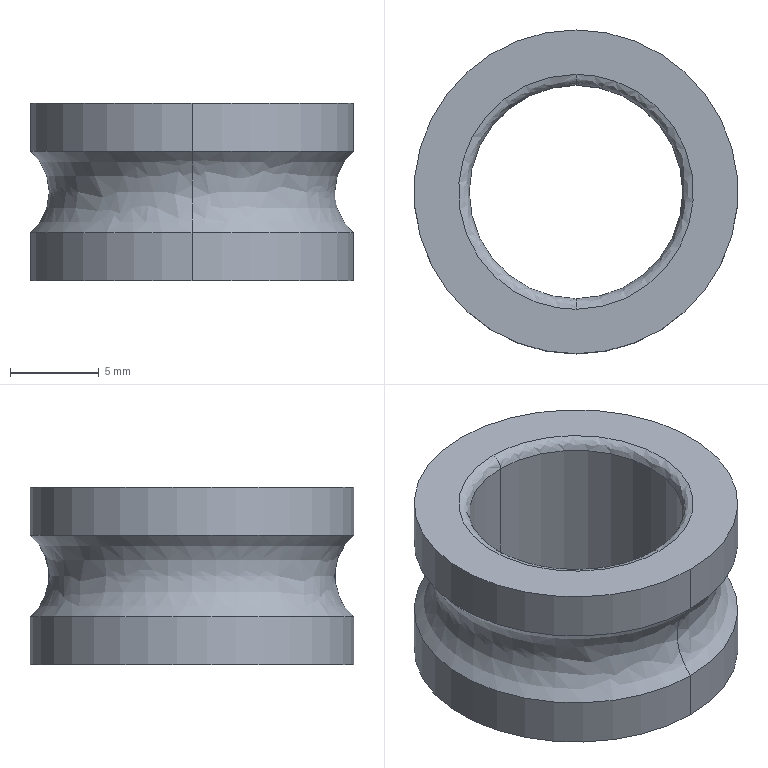Part | SolidWorks | features BaseBody 1 | 1 solid | 14 faces | box 18.2 x 18.2 x 10 mm | volume 1277 mm3 | spline 6 | cylinder 6 | plane 2 | commonest cylinder face diameters 18.2 x4 12 x2
STEP:
#1=CARTESIAN_POINT('',(0.,6.6,10.));
#2=VERTEX_POINT('',#1);
#3=CARTESIAN_POINT('',(0.,-6.6,10.));
#4=VERTEX_POINT('',#3);
#5=CARTESIAN_POINT('',(0.,6.6,10.));
#6=CARTESIAN_POINT('',(-13.2,6.6,10.));
#7=CARTESIAN_POINT('',(-13.2,-6.6,10.));
#8=CARTESIAN_POINT('',(0.,-6.6,10.));
#9=(BOUNDED_CURVE()B_SPLINE_CURVE(3,(#5,#6,#7,#8),.UNSPECIFIED.,.F.,.F.)B_SPLINE_CURVE_WITH_KNOTS((4,4),(0.25,0.75),.UNSPECIFIED.)CURVE()GEOMETRIC_REPRESENTATION_ITEM()RATIONAL_B_SPLINE_CURVE((1.,0.3333,0.3333,1.))REPRESENTATION_ITEM(''));
#10=EDGE_CURVE('',#2,#4,#9,.T.);
#11=ORIENTED_EDGE('',*,*,#10,.T.);
#12=CARTESIAN_POINT('',(0.,-6.,9.4));
#13=VERTEX_POINT('',#12);
#14=CARTESIAN_POINT('',(0.,-6.6,9.4));
#15=DIRECTION('',(-1.,0.,0.));
#16=DIRECTION('',(0.,-1.,0.));
#17=AXIS2_PLACEMENT_3D('',#14,#15,#16);
#18=CIRCLE('',#17,0.6);
#19=EDGE_CURVE('',#4,#13,#18,.T.);
#20=ORIENTED_EDGE('',*,*,#19,.T.);
#21=CARTESIAN_POINT('',(0.,6.,9.4));
#22=VERTEX_POINT('',#21);
#23=CARTESIAN_POINT('',(0.,0.,9.4));
#24=DIRECTION('',(0.,0.,-1.));
#25=DIRECTION('',(0.,1.,0.));
#26=AXIS2_PLACEMENT_3D('',#23,#24,#25);
#27=CIRCLE('',#26,6.);
#28=EDGE_CURVE('',#13,#22,#27,.T.);
#29=ORIENTED_EDGE('',*,*,#28,.T.);
#30=CARTESIAN_POINT('',(0.,6.6,9.4));
#31=DIRECTION('',(1.,0.,0.));
#32=DIRECTION('',(0.,1.,0.));
#33=AXIS2_PLACEMENT_3D('',#30,#31,#32);
#34=CIRCLE('',#33,0.6);
#35=EDGE_CURVE('',#2,#22,#34,.T.);
#36=ORIENTED_EDGE('',*,*,#35,.F.);
#37=EDGE_LOOP('',(#11,#20,#29,#36));
#38=FACE_OUTER_BOUND('',#37,.T.);
#39=CARTESIAN_POINT('',(0.,-6.6,10.));
#40=CARTESIAN_POINT('',(-13.2,-6.6,10.));
#41=CARTESIAN_POINT('',(-13.2,6.6,10.));
#42=CARTESIAN_POINT('',(0.,6.6,10.));
#43=CARTESIAN_POINT('',(0.,-6.249,10.));
#44=CARTESIAN_POINT('',(-12.497,-6.249,10.));
#45=CARTESIAN_POINT('',(-12.497,6.249,10.));
#46=CARTESIAN_POINT('',(0.,6.249,10.));
#47=CARTESIAN_POINT('',(0.,-6.,9.751));
#48=CARTESIAN_POINT('',(-12.,-6.,9.751));
#49=CARTESIAN_POINT('',(-12.,6.,9.751));
#50=CARTESIAN_POINT('',(0.,6.,9.751));
#51=CARTESIAN_POINT('',(0.,-6.,9.4));
#52=CARTESIAN_POINT('',(-12.,-6.,9.4));
#53=CARTESIAN_POINT('',(-12.,6.,9.4));
#54=CARTESIAN_POINT('',(0.,6.,9.4));
#55=(BOUNDED_SURFACE()B_SPLINE_SURFACE(3,3,((#39,#40,#41,#42),(#43,#44,#45,#46),(#47,#48,#49,#50),(#51,#52,#53,#54)),.UNSPECIFIED.,.F.,.F.,.F.)B_SPLINE_SURFACE_WITH_KNOTS((4,4),(4,4),(0.,1.),(0.,1.),.UNSPECIFIED.)GEOMETRIC_REPRESENTATION_ITEM()RATIONAL_B_SPLINE_SURFACE(((1.,0.3333,0.3333,1.),(0.8047,0.2682,0.2682,0.8047),(0.8047,0.2682,0.2682,0.8047),(1.,0.3333,0.3333,1.)))REPRESENTATION_ITEM('')SURFACE());
#56=ADVANCED_FACE('',(#38),#55,.T.);
#57=CARTESIAN_POINT('',(0.,6.,0.6));
#58=VERTEX_POINT('',#57);
#59=CARTESIAN_POINT('',(0.,-6.,0.6));
#60=VERTEX_POINT('',#59);
#61=CARTESIAN_POINT('',(0.,0.,0.6));
#62=DIRECTION('',(0.,0.,1.));
#63=DIRECTION('',(0.,1.,0.));
#64=AXIS2_PLACEMENT_3D('',#61,#62,#63);
#65=CIRCLE('',#64,6.);
#66=EDGE_CURVE('',#58,#60,#65,.T.);
#67=ORIENTED_EDGE('',*,*,#66,.T.);
#68=CARTESIAN_POINT('',(0.,-6.6,0.));
#69=VERTEX_POINT('',#68);
#70=CARTESIAN_POINT('',(0.,-6.6,0.6));
#71=DIRECTION('',(-1.,0.,0.));
#72=DIRECTION('',(0.,-1.,0.));
#73=AXIS2_PLACEMENT_3D('',#70,#71,#72);
#74=CIRCLE('',#73,0.6);
#75=EDGE_CURVE('',#60,#69,#74,.T.);
#76=ORIENTED_EDGE('',*,*,#75,.T.);
#77=CARTESIAN_POINT('',(0.,6.6,0.));
#78=VERTEX_POINT('',#77);
#79=CARTESIAN_POINT('',(0.,-6.6,0.));
#80=CARTESIAN_POINT('',(-13.2,-6.6,0.));
#81=CARTESIAN_POINT('',(-13.2,6.6,0.));
#82=CARTESIAN_POINT('',(0.,6.6,0.));
#83=(BOUNDED_CURVE()B_SPLINE_CURVE(3,(#79,#80,#81,#82),.UNSPECIFIED.,.F.,.T.)B_SPLINE_CURVE_WITH_KNOTS((4,4),(0.25,0.75),.UNSPECIFIED.)CURVE()GEOMETRIC_REPRESENTATION_ITEM()RATIONAL_B_SPLINE_CURVE((1.,0.3333,0.3333,1.))REPRESENTATION_ITEM(''));
#84=EDGE_CURVE('',#69,#78,#83,.T.);
#85=ORIENTED_EDGE('',*,*,#84,.T.);
#86=CARTESIAN_POINT('',(0.,6.6,0.6));
#87=DIRECTION('',(1.,0.,0.));
#88=DIRECTION('',(0.,1.,0.));
#89=AXIS2_PLACEMENT_3D('',#86,#87,#88);
#90=CIRCLE('',#89,0.6);
#91=EDGE_CURVE('',#58,#78,#90,.T.);
#92=ORIENTED_EDGE('',*,*,#91,.F.);
#93=EDGE_LOOP('',(#67,#76,#85,#92));
#94=FACE_OUTER_BOUND('',#93,.T.);
#95=CARTESIAN_POINT('',(0.,-6.,0.6));
#96=CARTESIAN_POINT('',(-12.,-6.,0.6));
#97=CARTESIAN_POINT('',(-12.,6.,0.6));
#98=CARTESIAN_POINT('',(0.,6.,0.6));
#99=CARTESIAN_POINT('',(0.,-6.,0.2485));
#100=CARTESIAN_POINT('',(-12.,-6.,0.2485));
#101=CARTESIAN_POINT('',(-12.,6.,0.2485));
#102=CARTESIAN_POINT('',(0.,6.,0.2485));
#103=CARTESIAN_POINT('',(0.,-6.249,0.));
#104=CARTESIAN_POINT('',(-12.497,-6.249,0.));
#105=CARTESIAN_POINT('',(-12.497,6.249,0.));
#106=CARTESIAN_POINT('',(0.,6.249,0.));
#107=CARTESIAN_POINT('',(0.,-6.6,0.));
#108=CARTESIAN_POINT('',(-13.2,-6.6,0.));
#109=CARTESIAN_POINT('',(-13.2,6.6,0.));
#110=CARTESIAN_POINT('',(0.,6.6,0.));
#111=(BOUNDED_SURFACE()B_SPLINE_SURFACE(3,3,((#95,#96,#97,#98),(#99,#100,#101,#102),(#103,#104,#105,#106),(#107,#108,#109,#110)),.UNSPECIFIED.,.F.,.F.,.T.)B_SPLINE_SURFACE_WITH_KNOTS((4,4),(4,4),(0.,1.),(0.,1.),.UNSPECIFIED.)GEOMETRIC_REPRESENTATION_ITEM()RATIONAL_B_SPLINE_SURFACE(((1.,0.3333,0.3333,1.),(0.8047,0.2682,0.2682,0.8047),(0.8047,0.2682,0.2682,0.8047),(1.,0.3333,0.3333,1.)))REPRESENTATION_ITEM('')SURFACE());
#112=ADVANCED_FACE('',(#94),#111,.T.);
#113=CARTESIAN_POINT('',(0.,-9.1,7.301));
#114=VERTEX_POINT('',#113);
#115=CARTESIAN_POINT('',(0.,9.1,7.301));
#116=VERTEX_POINT('',#115);
#117=CARTESIAN_POINT('',(0.,0.,7.301));
#118=DIRECTION('',(0.,0.,1.));
#119=DIRECTION('',(0.,1.,0.));
#120=AXIS2_PLACEMENT_3D('',#117,#118,#119);
#121=CIRCLE('',#120,9.1);
#122=EDGE_CURVE('',#114,#116,#121,.T.);
#123=ORIENTED_EDGE('',*,*,#122,.F.);
#124=CARTESIAN_POINT('',(0.,-9.1,2.699));
#125=VERTEX_POINT('',#124);
#126=CARTESIAN_POINT('',(0.,-11.025,5.));
#127=DIRECTION('',(-1.,0.,0.));
#128=DIRECTION('',(0.,-1.,0.));
#129=AXIS2_PLACEMENT_3D('',#126,#127,#128);
#130=CIRCLE('',#129,3.);
#131=EDGE_CURVE('',#114,#125,#130,.T.);
#132=ORIENTED_EDGE('',*,*,#131,.T.);
#133=CARTESIAN_POINT('',(0.,9.1,2.699));
#134=VERTEX_POINT('',#133);
#135=CARTESIAN_POINT('',(0.,0.,2.699));
#136=DIRECTION('',(0.,0.,-1.));
#137=DIRECTION('',(0.,1.,0.));
#138=AXIS2_PLACEMENT_3D('',#135,#136,#137);
#139=CIRCLE('',#138,9.1);
#140=EDGE_CURVE('',#134,#125,#139,.T.);
#141=ORIENTED_EDGE('',*,*,#140,.F.);
#142=CARTESIAN_POINT('',(0.,11.025,5.));
#143=DIRECTION('',(1.,0.,0.));
#144=DIRECTION('',(0.,1.,0.));
#145=AXIS2_PLACEMENT_3D('',#142,#143,#144);
#146=CIRCLE('',#145,3.);
#147=EDGE_CURVE('',#116,#134,#146,.T.);
#148=ORIENTED_EDGE('',*,*,#147,.F.);
#149=EDGE_LOOP('',(#123,#132,#141,#148));
#150=FACE_OUTER_BOUND('',#149,.T.);
#151=CARTESIAN_POINT('',(0.,9.1,7.301));
#152=CARTESIAN_POINT('',(18.2,9.1,7.301));
#153=CARTESIAN_POINT('',(18.2,-9.1,7.301));
#154=CARTESIAN_POINT('',(0.,-9.1,7.301));
#155=CARTESIAN_POINT('',(0.,7.554,6.008));
#156=CARTESIAN_POINT('',(15.108,7.554,6.008));
#157=CARTESIAN_POINT('',(15.108,-7.554,6.008));
#158=CARTESIAN_POINT('',(0.,-7.554,6.008));
#159=CARTESIAN_POINT('',(0.,7.554,3.992));
#160=CARTESIAN_POINT('',(15.108,7.554,3.992));
#161=CARTESIAN_POINT('',(15.108,-7.554,3.992));
#162=CARTESIAN_POINT('',(0.,-7.554,3.992));
#163=CARTESIAN_POINT('',(0.,9.1,2.699));
#164=CARTESIAN_POINT('',(18.2,9.1,2.699));
#165=CARTESIAN_POINT('',(18.2,-9.1,2.699));
#166=CARTESIAN_POINT('',(0.,-9.1,2.699));
#167=(BOUNDED_SURFACE()B_SPLINE_SURFACE(3,3,((#151,#152,#153,#154),(#155,#156,#157,#158),(#159,#160,#161,#162),(#163,#164,#165,#166)),.UNSPECIFIED.,.F.,.F.,.F.)B_SPLINE_SURFACE_WITH_KNOTS((4,4),(4,4),(0.,1.),(0.,1.),.UNSPECIFIED.)GEOMETRIC_REPRESENTATION_ITEM()RATIONAL_B_SPLINE_SURFACE(((1.,0.3333,0.3333,1.),(0.7611,0.2537,0.2537,0.7611),(0.7611,0.2537,0.2537,0.7611),(1.,0.3333,0.3333,1.)))REPRESENTATION_ITEM('')SURFACE());
#168=ADVANCED_FACE('',(#150),#167,.F.);
#169=ORIENTED_EDGE('',*,*,#28,.F.);
#170=CARTESIAN_POINT('',(0.,-6.,0.));
#171=DIRECTION('',(0.,0.,-1.));
#172=VECTOR('',#171,1000.);
#173=LINE('',#170,#172);
#174=EDGE_CURVE('',#13,#60,#173,.T.);
#175=ORIENTED_EDGE('',*,*,#174,.T.);
#176=ORIENTED_EDGE('',*,*,#66,.F.);
#177=CARTESIAN_POINT('',(0.,6.,0.));
#178=DIRECTION('',(0.,0.,-1.));
#179=VECTOR('',#178,1000.);
#180=LINE('',#177,#179);
#181=EDGE_CURVE('',#22,#58,#180,.T.);
#182=ORIENTED_EDGE('',*,*,#181,.F.);
#183=EDGE_LOOP('',(#169,#175,#176,#182));
#184=FACE_OUTER_BOUND('',#183,.T.);
#185=CARTESIAN_POINT('',(0.,0.,0.));
#186=DIRECTION('',(0.,0.,-1.));
#187=DIRECTION('',(0.,1.,0.));
#188=AXIS2_PLACEMENT_3D('',#185,#186,#187);
#189=CYLINDRICAL_SURFACE('',#188,6.);
#190=ADVANCED_FACE('',(#184),#189,.F.);
#191=CARTESIAN_POINT('',(0.,-9.1,10.));
#192=VERTEX_POINT('',#191);
#193=CARTESIAN_POINT('',(0.,9.1,10.));
#194=VERTEX_POINT('',#193);
#195=CARTESIAN_POINT('',(0.,0.,10.));
#196=DIRECTION('',(0.,0.,1.));
#197=DIRECTION('',(0.,1.,0.));
#198=AXIS2_PLACEMENT_3D('',#195,#196,#197);
#199=CIRCLE('',#198,9.1);
#200=EDGE_CURVE('',#192,#194,#199,.T.);
#201=ORIENTED_EDGE('',*,*,#200,.F.);
#202=CARTESIAN_POINT('',(0.,-9.1,0.));
#203=DIRECTION('',(0.,0.,-1.));
#204=VECTOR('',#203,1000.);
#205=LINE('',#202,#204);
#206=EDGE_CURVE('',#192,#114,#205,.T.);
#207=ORIENTED_EDGE('',*,*,#206,.T.);
#208=ORIENTED_EDGE('',*,*,#122,.T.);
#209=CARTESIAN_POINT('',(0.,9.1,0.));
#210=DIRECTION('',(0.,0.,-1.));
#211=VECTOR('',#210,1000.);
#212=LINE('',#209,#211);
#213=EDGE_CURVE('',#194,#116,#212,.T.);
#214=ORIENTED_EDGE('',*,*,#213,.F.);
#215=EDGE_LOOP('',(#201,#207,#208,#214));
#216=FACE_OUTER_BOUND('',#215,.T.);
#217=CARTESIAN_POINT('',(0.,0.,0.));
#218=DIRECTION('',(0.,0.,-1.));
#219=DIRECTION('',(0.,1.,0.));
#220=AXIS2_PLACEMENT_3D('',#217,#218,#219);
#221=CYLINDRICAL_SURFACE('',#220,9.1);
#222=ADVANCED_FACE('',(#216),#221,.T.);
#223=ORIENTED_EDGE('',*,*,#140,.T.);
#224=CARTESIAN_POINT('',(0.,-9.1,0.));
#225=VERTEX_POINT('',#224);
#226=CARTESIAN_POINT('',(0.,-9.1,0.));
#227=DIRECTION('',(0.,0.,-1.));
#228=VECTOR('',#227,1000.);
#229=LINE('',#226,#228);
#230=EDGE_CURVE('',#125,#225,#229,.T.);
#231=ORIENTED_EDGE('',*,*,#230,.T.);
#232=CARTESIAN_POINT('',(0.,9.1,0.));
#233=VERTEX_POINT('',#232);
#234=CARTESIAN_POINT('',(0.,0.,0.));
#235=DIRECTION('',(0.,0.,-1.));
#236=DIRECTION('',(0.,1.,0.));
#237=AXIS2_PLACEMENT_3D('',#234,#235,#236);
#238=CIRCLE('',#237,9.1);
#239=EDGE_CURVE('',#233,#225,#238,.T.);
#240=ORIENTED_EDGE('',*,*,#239,.F.);
#241=CARTESIAN_POINT('',(0.,9.1,0.));
#242=DIRECTION('',(0.,0.,-1.));
#243=VECTOR('',#242,1000.);
#244=LINE('',#241,#243);
#245=EDGE_CURVE('',#134,#233,#244,.T.);
#246=ORIENTED_EDGE('',*,*,#245,.F.);
#247=EDGE_LOOP('',(#223,#231,#240,#246));
#248=FACE_OUTER_BOUND('',#247,.T.);
#249=CARTESIAN_POINT('',(0.,0.,0.));
#250=DIRECTION('',(0.,0.,-1.));
#251=DIRECTION('',(0.,1.,0.));
#252=AXIS2_PLACEMENT_3D('',#249,#250,#251);
#253=CYLINDRICAL_SURFACE('',#252,9.1);
#254=ADVANCED_FACE('',(#248),#253,.T.);
#255=ORIENTED_EDGE('',*,*,#174,.F.);
#256=CARTESIAN_POINT('',(0.,0.,9.4));
#257=DIRECTION('',(0.,0.,-1.));
#258=DIRECTION('',(0.,1.,0.));
#259=AXIS2_PLACEMENT_3D('',#256,#257,#258);
#260=CIRCLE('',#259,6.);
#261=EDGE_CURVE('',#22,#13,#260,.T.);
#262=ORIENTED_EDGE('',*,*,#261,.F.);
#263=ORIENTED_EDGE('',*,*,#181,.T.);
#264=CARTESIAN_POINT('',(0.,0.,0.6));
#265=DIRECTION('',(0.,0.,1.));
#266=DIRECTION('',(0.,1.,0.));
#267=AXIS2_PLACEMENT_3D('',#264,#265,#266);
#268=CIRCLE('',#267,6.);
#269=EDGE_CURVE('',#60,#58,#268,.T.);
#270=ORIENTED_EDGE('',*,*,#269,.F.);
#271=EDGE_LOOP('',(#255,#262,#263,#270));
#272=FACE_OUTER_BOUND('',#271,.T.);
#273=CARTESIAN_POINT('',(0.,0.,0.));
#274=DIRECTION('',(0.,0.,-1.));
#275=DIRECTION('',(0.,1.,0.));
#276=AXIS2_PLACEMENT_3D('',#273,#274,#275);
#277=CYLINDRICAL_SURFACE('',#276,6.);
#278=ADVANCED_FACE('',(#272),#277,.F.);
#279=ORIENTED_EDGE('',*,*,#19,.F.);
#280=CARTESIAN_POINT('',(0.,-6.6,10.));
#281=CARTESIAN_POINT('',(13.2,-6.6,10.));
#282=CARTESIAN_POINT('',(13.2,6.6,10.));
#283=CARTESIAN_POINT('',(0.,6.6,10.));
#284=(BOUNDED_CURVE()B_SPLINE_CURVE(3,(#280,#281,#282,#283),.UNSPECIFIED.,.F.,.T.)B_SPLINE_CURVE_WITH_KNOTS((4,4),(0.75,1.25),.UNSPECIFIED.)CURVE()GEOMETRIC_REPRESENTATION_ITEM()RATIONAL_B_SPLINE_CURVE((1.,0.3333,0.3333,1.))REPRESENTATION_ITEM(''));
#285=EDGE_CURVE('',#4,#2,#284,.T.);
#286=ORIENTED_EDGE('',*,*,#285,.T.);
#287=ORIENTED_EDGE('',*,*,#35,.T.);
#288=ORIENTED_EDGE('',*,*,#261,.T.);
#289=EDGE_LOOP('',(#279,#286,#287,#288));
#290=FACE_OUTER_BOUND('',#289,.T.);
#291=CARTESIAN_POINT('',(0.,6.6,10.));
#292=CARTESIAN_POINT('',(13.2,6.6,10.));
#293=CARTESIAN_POINT('',(13.2,-6.6,10.));
#294=CARTESIAN_POINT('',(0.,-6.6,10.));
#295=CARTESIAN_POINT('',(0.,6.249,10.));
#296=CARTESIAN_POINT('',(12.497,6.249,10.));
#297=CARTESIAN_POINT('',(12.497,-6.249,10.));
#298=CARTESIAN_POINT('',(0.,-6.249,10.));
#299=CARTESIAN_POINT('',(0.,6.,9.751));
#300=CARTESIAN_POINT('',(12.,6.,9.751));
#301=CARTESIAN_POINT('',(12.,-6.,9.751));
#302=CARTESIAN_POINT('',(0.,-6.,9.751));
#303=CARTESIAN_POINT('',(0.,6.,9.4));
#304=CARTESIAN_POINT('',(12.,6.,9.4));
#305=CARTESIAN_POINT('',(12.,-6.,9.4));
#306=CARTESIAN_POINT('',(0.,-6.,9.4));
#307=(BOUNDED_SURFACE()B_SPLINE_SURFACE(3,3,((#291,#292,#293,#294),(#295,#296,#297,#298),(#299,#300,#301,#302),(#303,#304,#305,#306)),.UNSPECIFIED.,.F.,.F.,.F.)B_SPLINE_SURFACE_WITH_KNOTS((4,4),(4,4),(0.,1.),(0.,1.),.UNSPECIFIED.)GEOMETRIC_REPRESENTATION_ITEM()RATIONAL_B_SPLINE_SURFACE(((1.,0.3333,0.3333,1.),(0.8047,0.2682,0.2682,0.8047),(0.8047,0.2682,0.2682,0.8047),(1.,0.3333,0.3333,1.)))REPRESENTATION_ITEM('')SURFACE());
#308=ADVANCED_FACE('',(#290),#307,.T.);
#309=ORIENTED_EDGE('',*,*,#75,.F.);
#310=ORIENTED_EDGE('',*,*,#269,.T.);
#311=ORIENTED_EDGE('',*,*,#91,.T.);
#312=CARTESIAN_POINT('',(0.,6.6,0.));
#313=CARTESIAN_POINT('',(13.2,6.6,0.));
#314=CARTESIAN_POINT('',(13.2,-6.6,0.));
#315=CARTESIAN_POINT('',(0.,-6.6,0.));
#316=(BOUNDED_CURVE()B_SPLINE_CURVE(3,(#312,#313,#314,#315),.UNSPECIFIED.,.F.,.F.)B_SPLINE_CURVE_WITH_KNOTS((4,4),(0.75,1.25),.UNSPECIFIED.)CURVE()GEOMETRIC_REPRESENTATION_ITEM()RATIONAL_B_SPLINE_CURVE((1.,0.3333,0.3333,1.))REPRESENTATION_ITEM(''));
#317=EDGE_CURVE('',#78,#69,#316,.T.);
#318=ORIENTED_EDGE('',*,*,#317,.T.);
#319=EDGE_LOOP('',(#309,#310,#311,#318));
#320=FACE_OUTER_BOUND('',#319,.T.);
#321=CARTESIAN_POINT('',(0.,6.,0.6));
#322=CARTESIAN_POINT('',(12.,6.,0.6));
#323=CARTESIAN_POINT('',(12.,-6.,0.6));
#324=CARTESIAN_POINT('',(0.,-6.,0.6));
#325=CARTESIAN_POINT('',(0.,6.,0.2485));
#326=CARTESIAN_POINT('',(12.,6.,0.2485));
#327=CARTESIAN_POINT('',(12.,-6.,0.2485));
#328=CARTESIAN_POINT('',(0.,-6.,0.2485));
#329=CARTESIAN_POINT('',(0.,6.249,0.));
#330=CARTESIAN_POINT('',(12.497,6.249,0.));
#331=CARTESIAN_POINT('',(12.497,-6.249,0.));
#332=CARTESIAN_POINT('',(0.,-6.249,0.));
#333=CARTESIAN_POINT('',(0.,6.6,0.));
#334=CARTESIAN_POINT('',(13.2,6.6,0.));
#335=CARTESIAN_POINT('',(13.2,-6.6,0.));
#336=CARTESIAN_POINT('',(0.,-6.6,0.));
#337=(BOUNDED_SURFACE()B_SPLINE_SURFACE(3,3,((#321,#322,#323,#324),(#325,#326,#327,#328),(#329,#330,#331,#332),(#333,#334,#335,#336)),.UNSPECIFIED.,.F.,.F.,.F.)B_SPLINE_SURFACE_WITH_KNOTS((4,4),(4,4),(0.,1.),(0.,1.),.UNSPECIFIED.)GEOMETRIC_REPRESENTATION_ITEM()RATIONAL_B_SPLINE_SURFACE(((1.,0.3333,0.3333,1.),(0.8047,0.2682,0.2682,0.8047),(0.8047,0.2682,0.2682,0.8047),(1.,0.3333,0.3333,1.)))REPRESENTATION_ITEM('')SURFACE());
#338=ADVANCED_FACE('',(#320),#337,.T.);
#339=CARTESIAN_POINT('',(0.,0.,10.));
#340=DIRECTION('',(0.,0.,1.));
#341=DIRECTION('',(0.,1.,0.));
#342=AXIS2_PLACEMENT_3D('',#339,#340,#341);
#343=CIRCLE('',#342,9.1);
#344=EDGE_CURVE('',#194,#192,#343,.T.);
#345=ORIENTED_EDGE('',*,*,#344,.T.);
#346=ORIENTED_EDGE('',*,*,#200,.T.);
#347=EDGE_LOOP('',(#345,#346));
#348=FACE_OUTER_BOUND('',#347,.T.);
#349=ORIENTED_EDGE('',*,*,#10,.F.);
#350=ORIENTED_EDGE('',*,*,#285,.F.);
#351=EDGE_LOOP('',(#349,#350));
#352=FACE_BOUND('',#351,.T.);
#353=CARTESIAN_POINT('',(9.1,0.,10.));
#354=DIRECTION('',(0.,0.,1.));
#355=DIRECTION('',(0.,-1.,0.));
#356=AXIS2_PLACEMENT_3D('',#353,#354,#355);
#357=PLANE('',#356);
#358=ADVANCED_FACE('',(#348,#352),#357,.T.);
#359=ORIENTED_EDGE('',*,*,#317,.F.);
#360=ORIENTED_EDGE('',*,*,#84,.F.);
#361=EDGE_LOOP('',(#359,#360));
#362=FACE_BOUND('',#361,.T.);
#363=ORIENTED_EDGE('',*,*,#239,.T.);
#364=CARTESIAN_POINT('',(0.,0.,0.));
#365=DIRECTION('',(0.,0.,-1.));
#366=DIRECTION('',(0.,1.,0.));
#367=AXIS2_PLACEMENT_3D('',#364,#365,#366);
#368=CIRCLE('',#367,9.1);
#369=EDGE_CURVE('',#225,#233,#368,.T.);
#370=ORIENTED_EDGE('',*,*,#369,.T.);
#371=EDGE_LOOP('',(#363,#370));
#372=FACE_OUTER_BOUND('',#371,.T.);
#373=CARTESIAN_POINT('',(6.6,0.,0.));
#374=DIRECTION('',(0.,0.,-1.));
#375=DIRECTION('',(0.,1.,0.));
#376=AXIS2_PLACEMENT_3D('',#373,#374,#375);
#377=PLANE('',#376);
#378=ADVANCED_FACE('',(#362,#372),#377,.T.);
#379=ORIENTED_EDGE('',*,*,#206,.F.);
#380=ORIENTED_EDGE('',*,*,#344,.F.);
#381=ORIENTED_EDGE('',*,*,#213,.T.);
#382=CARTESIAN_POINT('',(0.,0.,7.301));
#383=DIRECTION('',(0.,0.,1.));
#384=DIRECTION('',(0.,1.,0.));
#385=AXIS2_PLACEMENT_3D('',#382,#383,#384);
#386=CIRCLE('',#385,9.1);
#387=EDGE_CURVE('',#116,#114,#386,.T.);
#388=ORIENTED_EDGE('',*,*,#387,.T.);
#389=EDGE_LOOP('',(#379,#380,#381,#388));
#390=FACE_OUTER_BOUND('',#389,.T.);
#391=CARTESIAN_POINT('',(0.,0.,0.));
#392=DIRECTION('',(0.,0.,-1.));
#393=DIRECTION('',(0.,1.,0.));
#394=AXIS2_PLACEMENT_3D('',#391,#392,#393);
#395=CYLINDRICAL_SURFACE('',#394,9.1);
#396=ADVANCED_FACE('',(#390),#395,.T.);
#397=ORIENTED_EDGE('',*,*,#230,.F.);
#398=CARTESIAN_POINT('',(0.,0.,2.699));
#399=DIRECTION('',(0.,0.,-1.));
#400=DIRECTION('',(0.,1.,0.));
#401=AXIS2_PLACEMENT_3D('',#398,#399,#400);
#402=CIRCLE('',#401,9.1);
#403=EDGE_CURVE('',#125,#134,#402,.T.);
#404=ORIENTED_EDGE('',*,*,#403,.T.);
#405=ORIENTED_EDGE('',*,*,#245,.T.);
#406=ORIENTED_EDGE('',*,*,#369,.F.);
#407=EDGE_LOOP('',(#397,#404,#405,#406));
#408=FACE_OUTER_BOUND('',#407,.T.);
#409=CARTESIAN_POINT('',(0.,0.,0.));
#410=DIRECTION('',(0.,0.,-1.));
#411=DIRECTION('',(0.,1.,0.));
#412=AXIS2_PLACEMENT_3D('',#409,#410,#411);
#413=CYLINDRICAL_SURFACE('',#412,9.1);
#414=ADVANCED_FACE('',(#408),#413,.T.);
#415=ORIENTED_EDGE('',*,*,#131,.F.);
#416=ORIENTED_EDGE('',*,*,#387,.F.);
#417=ORIENTED_EDGE('',*,*,#147,.T.);
#418=ORIENTED_EDGE('',*,*,#403,.F.);
#419=EDGE_LOOP('',(#415,#416,#417,#418));
#420=FACE_OUTER_BOUND('',#419,.T.);
#421=CARTESIAN_POINT('',(0.,-9.1,7.301));
#422=CARTESIAN_POINT('',(-18.2,-9.1,7.301));
#423=CARTESIAN_POINT('',(-18.2,9.1,7.301));
#424=CARTESIAN_POINT('',(0.,9.1,7.301));
#425=CARTESIAN_POINT('',(0.,-7.554,6.008));
#426=CARTESIAN_POINT('',(-15.108,-7.554,6.008));
#427=CARTESIAN_POINT('',(-15.108,7.554,6.008));
#428=CARTESIAN_POINT('',(0.,7.554,6.008));
#429=CARTESIAN_POINT('',(0.,-7.554,3.992));
#430=CARTESIAN_POINT('',(-15.108,-7.554,3.992));
#431=CARTESIAN_POINT('',(-15.108,7.554,3.992));
#432=CARTESIAN_POINT('',(0.,7.554,3.992));
#433=CARTESIAN_POINT('',(0.,-9.1,2.699));
#434=CARTESIAN_POINT('',(-18.2,-9.1,2.699));
#435=CARTESIAN_POINT('',(-18.2,9.1,2.699));
#436=CARTESIAN_POINT('',(0.,9.1,2.699));
#437=(BOUNDED_SURFACE()B_SPLINE_SURFACE(3,3,((#421,#422,#423,#424),(#425,#426,#427,#428),(#429,#430,#431,#432),(#433,#434,#435,#436)),.UNSPECIFIED.,.F.,.F.,.T.)B_SPLINE_SURFACE_WITH_KNOTS((4,4),(4,4),(0.,1.),(0.,1.),.UNSPECIFIED.)GEOMETRIC_REPRESENTATION_ITEM()RATIONAL_B_SPLINE_SURFACE(((1.,0.3333,0.3333,1.),(0.7611,0.2537,0.2537,0.7611),(0.7611,0.2537,0.2537,0.7611),(1.,0.3333,0.3333,1.)))REPRESENTATION_ITEM('')SURFACE());
#438=ADVANCED_FACE('',(#420),#437,.F.);
#439=CLOSED_SHELL('',(#56,#112,#168,#190,#222,#254,#278,#308,#338,#358,#378,#396,#414,#438));
#440=MANIFOLD_SOLID_BREP('',#439);
#441=CARTESIAN_POINT('',(0.,0.,0.));
#442=DIRECTION('',(0.,0.,1.));
#443=DIRECTION('',(1.,0.,0.));
#444=AXIS2_PLACEMENT_3D('',#441,#442,#443);
#445=(LENGTH_UNIT()NAMED_UNIT(*)SI_UNIT(.MILLI.,.METRE.));
#446=UNCERTAINTY_MEASURE_WITH_UNIT(LENGTH_MEASURE(0.00001),#445,'','');
#447=(NAMED_UNIT(*)PLANE_ANGLE_UNIT()SI_UNIT($,.RADIAN.));
#448=(NAMED_UNIT(*)SI_UNIT($,.STERADIAN.)SOLID_ANGLE_UNIT());
#449=(GEOMETRIC_REPRESENTATION_CONTEXT(3)GLOBAL_UNCERTAINTY_ASSIGNED_CONTEXT((#446))GLOBAL_UNIT_ASSIGNED_CONTEXT((#445,#447,#448))REPRESENTATION_CONTEXT('',''));
#450=ADVANCED_BREP_SHAPE_REPRESENTATION('',(#440,#444),#449);